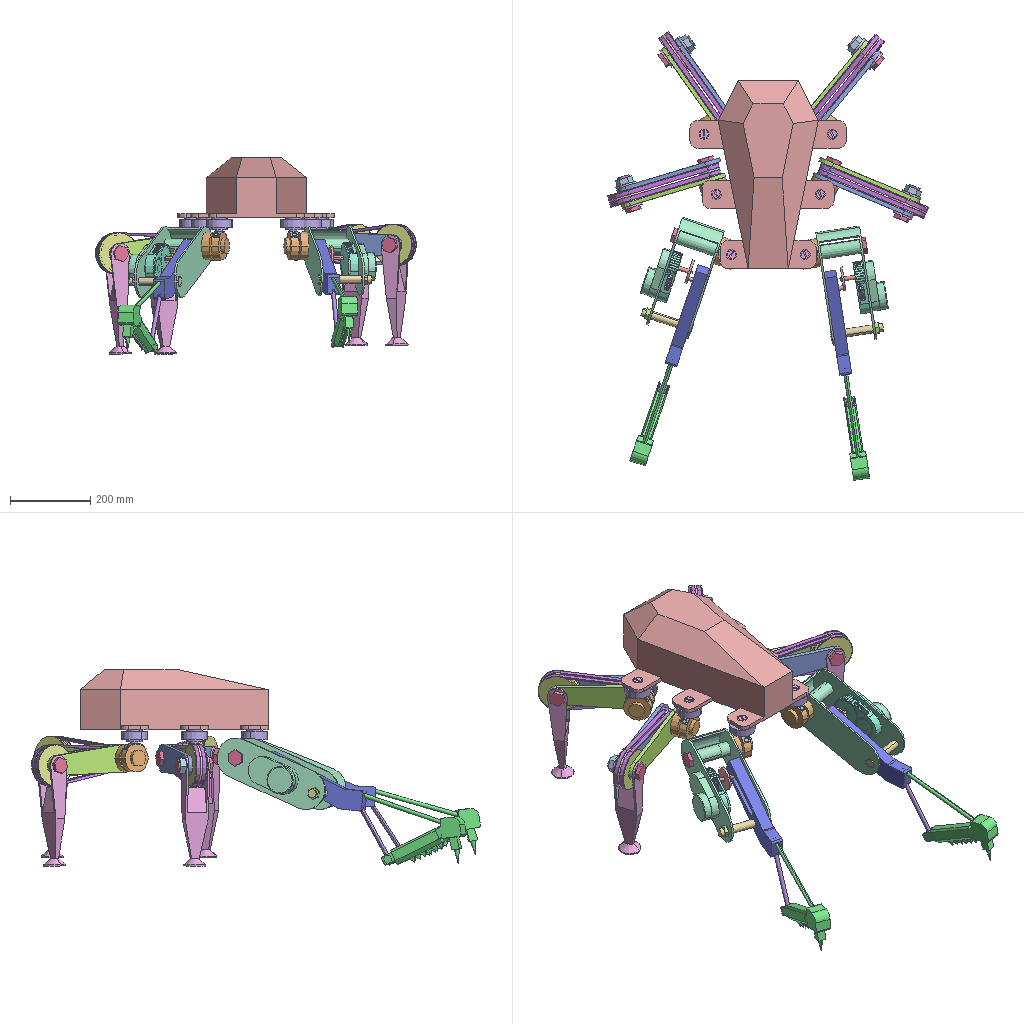Assembly | SolidWorks | 29 different items | 99 placed | box 801 x 1120 x 491 mm
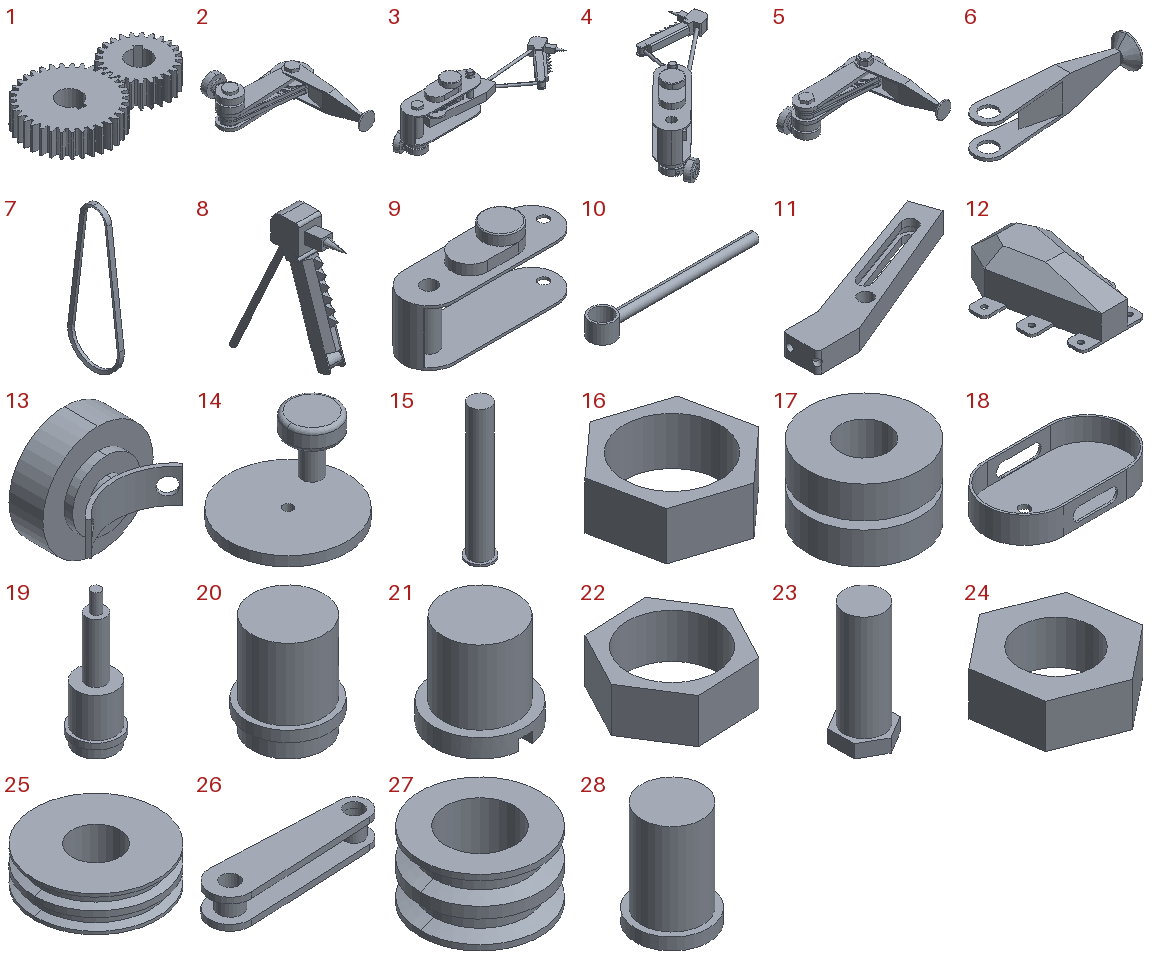Parts list (item | name | quantity | parent item | size | volume | features):
1 | (subassembly) | x2 | in 3, 4 | 123.948 x 73.952 x 20 mm | 100534 mm3 | features RefAxis 2
2 | (subassembly) | x2 | - | 297 x 321.802 x 142.5 mm | 1183355 mm3 | features CompositeCurve 2
3 | (subassembly) | x1 | - | 668.994 x 181.738 x 217.5 mm | 1662687 mm3 | -
4 | (subassembly) | x1 | - | 522.188 x 513.353 x 217.5 mm | 1544826 mm3 | -
5 | (subassembly) | x2 | - | 302.128 x 317.433 x 142.5 mm | 1183356 mm3 | features CompositeCurve 1
6 | - | x4 | in 2, 5 | 275.852 x 55.99 x 60 mm | 229238 mm3 | features ICE 3, Extrusion 1, Fillet 1, Revolution 1
7 | - | x8 | in 2, 5 | 10 x 103.625 x 288.63 mm | 30426 mm3 | features Sweep 1
8 | - | x2 | in 3, 4 | 40 x 207.302 x 265.068 mm | 279410 mm3 | features ICE 8, Fillet 5, Revolution 2, Extrusion 1
9 | - | x2 | in 3, 4 | 300 x 100 x 150 mm | 561268 mm3 | features ICE 7, Extrusion 1, Fillet 1
10 | - | x2 | in 3, 4 | 162 x 24 x 18 mm | 13348 mm3 | features Extrusion 1, ICE 1
11 | - | x2 | in 3, 4 | 264.316 x 123.025 x 30 mm | 276042 mm3 | features ICE 8, Fillet 2, Extrusion 1
12 | - | x1 | - | 390 x 470 x 150 mm | 2183743 mm3 | features ICE 16, Fillet 3, Extrusion 1, MirrorPattern 1, Shell 1
13 | - | x6 | in 2, 3, 4, 5 | 65 x 48.002 x 65 mm | 76467 mm3 | features ICE 5, RevCut 2, Extrusion 1
14 | - | x2 | in 3, 4 | 63.316 x 60 x 33 mm | 20231 mm3 | features ICE 3, Extrusion 1, Fillet 1
15 | - | x2 | in 3, 4 | 25 x 25 x 132 mm | 41822 mm3 | features Extrusion 1, ICE 1
16 | - | x2 | in 3, 4 | 27.456 x 28.236 x 10 mm | 2271 mm3 | features Extrusion 1
17 | - | x6 | in 2, 3, 4, 5 | 70 x 70 x 55 mm | 152574 mm3 | features ICE 3, RevCut 2, Extrusion 1
18 | - | x2 | in 3 | 135 x 75 x 25 mm | 48002 mm3 | features ICE 2, Extrusion 1, MirrorPattern 1
19 | - | x2 | in 3, 4 | 23 x 23 x 68 mm | 11653 mm3 | features ICE 4, Extrusion 1
20 | - | x2 | in 3, 4 | 23 x 23 x 28 mm | 9100 mm3 | features ICE 2, Extrusion 1
21 | - | x6 | - | 25 x 25 x 25 mm | 8464 mm3 | features ICE 2, Extrusion 1
22 | - | x4 | in 2, 5 | 42.69 x 37.825 x 15 mm | 7181 mm3 | features Extrusion 1
23 | - | x10 | in 2, 3, 5 | 35.299 x 40.41 x 90 mm | 67157 mm3 | features Extrusion 1, ICE 1
24 | - | x1 | in 4 | 8.601 x 9.134 x 3 mm | 107.372 mm3 | features Extrusion 1
25 | - | x4 | in 2, 5 | 104 x 104 x 30 mm | 188105 mm3 | features Extrusion 1, RevCut 1
26 | - | x4 | in 2, 5 | 270 x 70 x 50 mm | 300062 mm3 | features ICE 4, Extrusion 1
27 | - | x4 | in 2, 5 | 54 x 54 x 30 mm | 31755 mm3 | features Extrusion 1, RevCut 1
28 | - | x12 | in 2, 3, 5 | 12 x 12 x 17 mm | 1404 mm3 | features Extrusion 1, ICE 1
29 | spur gear_gb | x1 | - | - | - | -
Mates (type | each side: item.copy, entity, surface, feature):
In the top assembly
Concentric | 12.1 face cylinder Boss-Extrude4 | 13.1 face cylinder Cut-Extrude3
Concentric | 12.1 face cylinder Boss-Extrude4 | 13.2 face cylinder Cut-Extrude3
Concentric | 17.1 face cylinder Cut-Revolve2 | 28.1 face cylinder Boss-Extrude2
Tangent | 13.3 face cylinder Boss-Extrude4 | 28.1 face plane Boss-Extrude1
Concentric | 17.1 face cylinder Cut-Revolve3 | 28.2 face cylinder Boss-Extrude2
Tangent | 13.3 face cylinder Boss-Extrude4 | 28.2 edge
Concentric | 12.1 face cylinder Boss-Extrude4 | 21.1 face cylinder Boss-Extrude2
Concentric | 12.1 face cylinder Mirror1 | 21.2 face cylinder Boss-Extrude2
Concentric | 13.2 face cylinder Cut-Extrude3 | 21.3 face cylinder Boss-Extrude2
Concentric | 12.1 face cylinder Boss-Extrude4 | 21.4 face cylinder Boss-Extrude2
Concentric | 9.1 face cylinder Boss-Extrude2 | 23.1 face cylinder Boss-Extrude2
Coincident | 9.1 face plane Boss-Extrude3 | 23.1 face plane Boss-Extrude1
Coincident | 19.1 face cylinder Boss-Extrude4 | 18.1 edge
Coincident | 9.1 face plane Boss-Extrude3 | 18.1 face plane Boss-Extrude1
Concentric | 20.1 edge | 18.1 face cylinder Boss-Extrude1
Concentric | 21.2 face cylinder Boss-Extrude2 | 13.4 face cylinder Cut-Extrude3
Concentric | 21.5 face cylinder Boss-Extrude2 | 13.5 face cylinder Cut-Extrude3 | 2 times
Concentric | 12.1 face cylinder Mirror1 | 21.5 face cylinder Boss-Extrude2
Concentric | 12.1 face cylinder Mirror1 | 13.6 face cylinder Cut-Extrude3
Concentric | 13.6 face cylinder Cut-Extrude3 | 21.6 face cylinder Boss-Extrude2
Coincident | 12.1 face plane Cut-Extrude3 | 21.5 face plane Boss-Extrude1
Coincident | 12.1 face plane Boss-Extrude2 | 13.5 face plane Boss-Extrude8
Coincident | 12.1 face plane Cut-Extrude4 | 21.2 face plane Boss-Extrude1
Coincident | 12.1 face plane Boss-Extrude2 | 13.4 face plane Boss-Extrude8
Coincident | 12.1 face plane Cut-Extrude5 | 21.6 face plane Boss-Extrude1
Coincident | 12.1 face plane Boss-Extrude2 | 13.6 face plane Boss-Extrude8
Coincident | 12.1 face plane Cut-Extrude6 | 21.4 edge
Coincident | 12.1 face plane Boss-Extrude2 | 13.1 edge
Coincident | 12.1 face plane Cut-Extrude7 | 21.3 face plane Boss-Extrude1
Coincident | 12.1 face plane Boss-Extrude2 | 13.2 face plane Boss-Extrude8
Coincident | 12.1 face plane Cut-Extrude8 | 21.1 face plane Boss-Extrude1
Coincident | 12.1 face plane Boss-Extrude2 | 13.3 face plane Boss-Extrude8 | 2 times
Concentric | 13.3 face cylinder Cut-Extrude3 | 21.1 face cylinder Boss-Extrude2
In subassembly 2
Coincident | 26.1 face plane Boss-Extrude1 | 6.1 face plane Boss-Extrude8
Concentric | 26.1 face cylinder Boss-Extrude2 | 6.1 face cylinder Boss-Extrude8
Coincident | 26.1 face plane Boss-Extrude1 | 27.1 face plane Boss-Extrude1
Concentric | 26.1 face cylinder Boss-Extrude2 | 27.1 face cylinder Boss-Extrude1
Concentric | 17.2 face cylinder Boss-Extrude3 | 13.7 face cylinder Boss-Extrude4
Concentric | 17.2 face cylinder Cut-Revolve2 | 13.7 face cylinder Cut-Revolve3
Coincident | 17.2 face plane Boss-Extrude1 | 26.1 face plane Boss-Extrude1
Concentric | 26.1 face cylinder Cut-Extrude2 | 17.2 face cylinder Boss-Extrude1
Concentric | 13.7 face cylinder Cut-Revolve3 | 28.3 face cylinder Boss-Extrude2
Tangent | 13.7 face cylinder Boss-Extrude4 | 28.3 face plane Boss-Extrude1
Concentric | 17.2 face cylinder Cut-Revolve3 | 28.4 face cylinder Boss-Extrude2
Tangent | 13.7 face cylinder Boss-Extrude4 | 28.4 face plane Boss-Extrude1
Concentric | 26.1 face cylinder Boss-Extrude2 | 23.2 face cylinder Boss-Extrude2
Coincident | 6.1 face plane Boss-Extrude8 | 23.2 face plane Boss-Extrude1
Concentric | 23.2 face cylinder Boss-Extrude2 | 22.1 face cylinder Boss-Extrude1
Coincident | 6.1 face plane Boss-Extrude6 | 22.1 face plane Boss-Extrude1
Concentric | 26.1 face cylinder Cut-Extrude2 | 23.3 face cylinder Boss-Extrude2
Coincident | 26.1 face plane Boss-Extrude3 | 23.3 face plane Boss-Extrude1
Concentric | 26.1 face cylinder Boss-Extrude2 | 25.1 face cylinder Boss-Extrude1
Width | 25.1 face plane Boss-Extrude1 | 25.1 face plane Boss-Extrude1 | 26.1 face plane Boss-Extrude3 | 26.1 face plane Boss-Extrude1
Concentric | 25.1 face cylinder Cut-Revolve1 | 7.1 face cylinder Sweep1
Concentric | 27.1 face cylinder Cut-Revolve1 | 7.1 face cylinder Sweep1
Concentric | 25.1 face cylinder Cut-Revolve1 | 7.2 face cylinder Sweep1
Concentric | 27.1 face cylinder Cut-Revolve1 | 7.2 face cylinder Sweep1
In subassembly 5
Concentric | 26.1 face cylinder Boss-Extrude2 | 6.1 face cylinder Boss-Extrude8
Width | 6.1 face plane Boss-Extrude6 | 6.1 face plane Boss-Extrude8 | 26.1 face plane Boss-Extrude3 | 26.1 face plane Boss-Extrude1
Width | 25.2 face plane Boss-Extrude1 | 25.2 face plane Boss-Extrude1 | 26.1 face plane Boss-Extrude3 | 26.1 face plane Boss-Extrude1
Concentric | 25.2 face cylinder Boss-Extrude1 | 26.1 face cylinder Boss-Extrude2
Concentric | 26.1 face cylinder Boss-Extrude2 | 27.2 face cylinder Boss-Extrude1
Width | 27.2 face plane Boss-Extrude1 | 27.2 face plane Boss-Extrude1 | 26.1 face plane Boss-Extrude3 | 26.1 face plane Boss-Extrude1
Concentric | 27.2 face cylinder Cut-Revolve1 | 7.3 face cylinder Sweep1
Concentric | 25.2 face cylinder Cut-Revolve1 | 7.3 face cylinder Sweep1
Concentric | 25.2 face cylinder Cut-Revolve1 | 7.1 edge
Concentric | 27.2 face cylinder Cut-Revolve1 | 7.1 face cylinder Sweep1
Concentric | 26.1 face cylinder Boss-Extrude2 | 17.3 face cylinder Boss-Extrude1
Coincident | 26.1 face plane Boss-Extrude3 | 17.3 face plane Boss-Extrude1
Concentric | 13.8 face cylinder Boss-Extrude4 | 17.3 face cylinder Boss-Extrude3
Concentric | 13.8 face cylinder Cut-Revolve4 | 17.3 face cylinder Cut-Revolve3
Concentric | 26.1 face cylinder Cut-Extrude2 | 23.2 face cylinder Boss-Extrude2
Coincident | 6.1 face plane Boss-Extrude6 | 23.2 face plane Boss-Extrude1
Concentric | 22.2 face cylinder Boss-Extrude1 | 23.2 face cylinder Boss-Extrude2
Coincident | 6.1 face plane Boss-Extrude8 | 22.2 face plane Boss-Extrude1
Concentric | 26.1 face cylinder Boss-Extrude2 | 23.3 face cylinder Boss-Extrude2
Coincident | 26.1 face plane Boss-Extrude1 | 23.3 face plane Boss-Extrude1
Concentric | 17.3 face cylinder Cut-Revolve3 | 28.5 face cylinder Boss-Extrude2
Tangent | 13.8 face cylinder Boss-Extrude4 | 28.5 face plane Boss-Extrude1
Concentric | 17.3 face cylinder Cut-Revolve2 | 28.6 face cylinder Boss-Extrude2
Tangent | 13.8 face cylinder Boss-Extrude4 | 28.6 face plane Boss-Extrude1
In subassembly 4
Concentric | 9.2 face cylinder Cut-Extrude1 | 19.2 face cylinder Boss-Extrude1
Coincident | 9.2 face plane Boss-Extrude5 | 19.2 face plane Boss-Extrude1
Concentric | 9.2 face cylinder Cut-Extrude1 | 20.2 face cylinder Boss-Extrude2
Coincident | 9.2 face plane Boss-Extrude5 | 20.2 face plane Boss-Extrude2
Parallel | 9.2 face plane Boss-Extrude2 | 11.1 face plane Boss-Extrude1
Concentric | 9.2 face cylinder Cut-Extrude2 | 11.1 face cylinder Cut-Extrude3 | 2 times
Concentric | 11.1 face cylinder Cut-Extrude3 | 15.1 face cylinder Boss-Extrude7 | 2 times
Coincident | 9.2 face plane Boss-Extrude2 | 15.1 face plane Boss-Extrude1
Concentric | 11.1 face cylinder Cut-Extrude1 | 10.1 face cylinder Boss-Extrude2
Coincident | 11.1 face plane Cut-Extrude1 | 10.1 face plane Boss-Extrude2
Concentric | 10.1 face cylinder Boss-Extrude1 | 8.1 face cylinder Boss-Extrude16
Width | 8.1 face plane Boss-Extrude15 | 8.1 face plane Boss-Extrude15 | 10.1 face plane Boss-Extrude1 | 10.1 face plane Boss-Extrude1
Width | 8.1 face plane Boss-Extrude6 | 8.1 face plane Boss-Extrude6 | 11.1 face plane Boss-Extrude1 | 11.1 face plane Boss-Extrude1
Coincident | 9.2 face plane Boss-Extrude2 | 17.3 face plane Boss-Extrude1
Concentric | 9.2 face cylinder Boss-Extrude2 | 17.3 face cylinder Boss-Extrude1
Concentric | 17.3 face cylinder Boss-Extrude3 | 13.8 face cylinder Boss-Extrude4
Concentric | 17.3 face cylinder Cut-Revolve3 | 13.8 face cylinder Cut-Revolve4
Coincident | 9.2 face plane Boss-Extrude2 | 11.1 face plane Boss-Extrude1
Concentric | 19.2 face cylinder Boss-Extrude5 | 14.1 face cylinder Cut-Extrude1
Coincident | 19.2 face plane Boss-Extrude4 | 14.1 face plane Boss-Extrude1
Tangent | 11.1 face plane Cut-Extrude4 | 14.1 face cylinder Boss-Extrude3
Concentric | 19.2 face cylinder Boss-Extrude5 | 24.1 face cylinder Boss-Extrude1
Coincident | 14.1 face plane Boss-Extrude1 | 24.1 face plane Boss-Extrude1
Concentric | 15.1 face cylinder Boss-Extrude7 | 16.1 face cylinder Boss-Extrude1
Coincident | 9.2 face plane Boss-Extrude3 | 16.1 face plane Boss-Extrude1
In subassembly 3
Concentric | 9.2 face cylinder Cut-Extrude1 | 19.2 face cylinder Boss-Extrude1
Coincident | 9.2 face plane Boss-Extrude5 | 19.2 face plane Boss-Extrude1
Concentric | 9.2 face cylinder Cut-Extrude1 | 20.2 face cylinder Boss-Extrude2
Coincident | 9.2 face plane Boss-Extrude5 | 20.2 face plane Boss-Extrude2
Concentric | 19.2 face cylinder Boss-Extrude5 | 14.2 face cylinder Cut-Extrude1
Coincident | 19.2 face plane Boss-Extrude4 | 14.2 face plane Boss-Extrude1
Concentric | 9.2 face cylinder Cut-Extrude2 | 11.1 face cylinder Cut-Extrude3
Coincident | 9.2 face plane Boss-Extrude2 | 11.1 face plane Boss-Extrude1
Concentric | 14.2 face cylinder Boss-Extrude3 | 11.1 face cylinder Cut-Extrude4
Concentric | 9.2 face cylinder Cut-Extrude2 | 15.2 face cylinder Boss-Extrude7
Coincident | 9.2 face plane Boss-Extrude2 | 15.2 face plane Boss-Extrude1
Concentric | 19.2 face cylinder Boss-Extrude4 | 18.1 face cylinder Boss-Extrude1
Coincident | 9.2 face plane Boss-Extrude3 | 18.1 face plane Boss-Extrude1
Concentric | 20.2 face cylinder Boss-Extrude4 | 18.1 face cylinder Boss-Extrude1
Concentric | 11.1 face cylinder Cut-Extrude1 | 10.1 face cylinder Boss-Extrude2
Coincident | 11.1 face plane Cut-Extrude1 | 10.1 face plane Boss-Extrude2
Concentric | 8.2 face cylinder Boss-Extrude16 | 10.1 face cylinder Boss-Extrude1
Width | 10.1 face plane Boss-Extrude1 | 10.1 face plane Boss-Extrude1 | 8.2 face plane Boss-Extrude15 | 8.2 face plane Boss-Extrude15
Parallel | 11.1 face plane Boss-Extrude1 | 8.2 face plane Boss-Extrude6
Concentric | 9.2 face cylinder Boss-Extrude2 | 17.3 face cylinder Boss-Extrude1
Coincident | 9.2 face plane Boss-Extrude2 | 17.3 face plane Boss-Extrude1
Concentric | 13.8 face cylinder Cut-Revolve4 | 17.3 face cylinder Cut-Revolve3
Concentric | 13.8 face cylinder Boss-Extrude4 | 17.3 face cylinder Boss-Extrude3
Concentric | 9.2 face cylinder Boss-Extrude2 | 23.2 face cylinder Boss-Extrude2
Coincident | 9.2 face plane Boss-Extrude3 | 23.2 face plane Boss-Extrude1
Concentric | 17.3 face cylinder Cut-Revolve3 | 28.4 face cylinder Boss-Extrude2
Tangent | 13.8 face cylinder Boss-Extrude4 | 28.4 face plane Boss-Extrude1
Concentric | 17.3 face cylinder Cut-Revolve2 | 28.3 face cylinder Boss-Extrude2
Tangent | 13.8 face cylinder Boss-Extrude4 | 28.3 face plane Boss-Extrude1
Concentric | 15.2 face cylinder Boss-Extrude7 | 16.1 face cylinder Boss-Extrude1
Coincident | 9.2 face plane Boss-Extrude3 | 16.1 face plane Boss-Extrude1